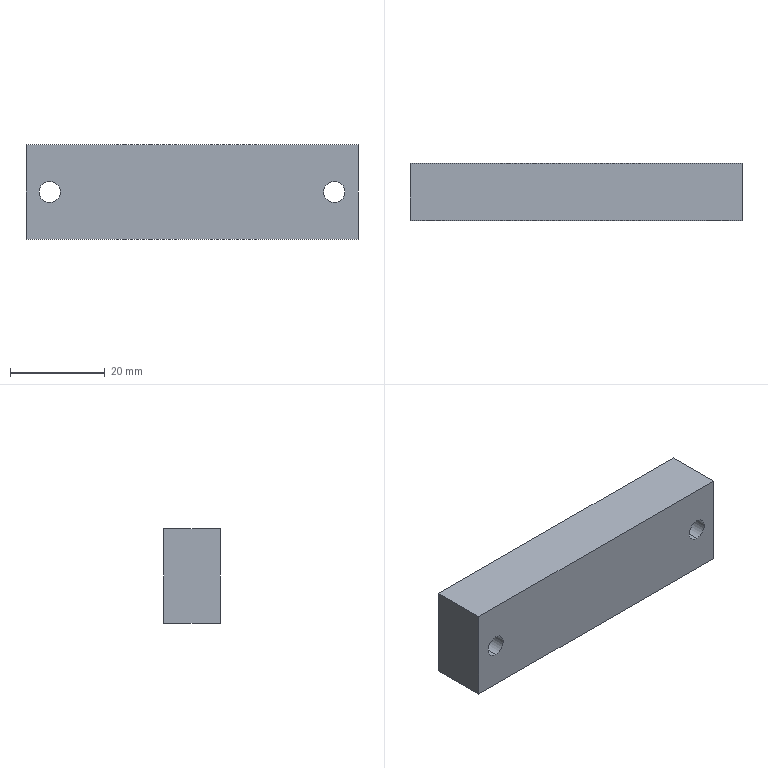Part | SolidWorks | features Extrusion 1, HoleWzd 1 | 1 solid | 16 faces | box 70 x 12 x 20 mm | volume 16291 mm3 | cylinder 8 | plane 8 | commonest cylinder face diameters 4.5 x4 7.8 x4
STEP:
#1=CARTESIAN_POINT('',(-30.,10.,-3.9));
#2=VERTEX_POINT('',#1);
#3=CARTESIAN_POINT('',(-30.,10.,3.9));
#4=VERTEX_POINT('',#3);
#5=CARTESIAN_POINT('',(-30.,10.,0.));
#6=DIRECTION('',(0.,1.,0.));
#7=DIRECTION('',(0.,0.,1.));
#8=AXIS2_PLACEMENT_3D('',#5,#6,#7);
#9=CIRCLE('',#8,3.9);
#10=EDGE_CURVE('',#2,#4,#9,.T.);
#11=ORIENTED_EDGE('',*,*,#10,.F.);
#12=CARTESIAN_POINT('',(-30.,12.,-3.9));
#13=VERTEX_POINT('',#12);
#14=CARTESIAN_POINT('',(-30.,12.,-3.9));
#15=DIRECTION('',(0.,1.,0.));
#16=VECTOR('',#15,1000.);
#17=LINE('',#14,#16);
#18=EDGE_CURVE('',#2,#13,#17,.T.);
#19=ORIENTED_EDGE('',*,*,#18,.T.);
#20=CARTESIAN_POINT('',(-30.,12.,3.9));
#21=VERTEX_POINT('',#20);
#22=CARTESIAN_POINT('',(-30.,12.,0.));
#23=DIRECTION('',(0.,1.,0.));
#24=DIRECTION('',(0.,0.,1.));
#25=AXIS2_PLACEMENT_3D('',#22,#23,#24);
#26=CIRCLE('',#25,3.9);
#27=EDGE_CURVE('',#13,#21,#26,.T.);
#28=ORIENTED_EDGE('',*,*,#27,.T.);
#29=CARTESIAN_POINT('',(-30.,12.,3.9));
#30=DIRECTION('',(0.,1.,0.));
#31=VECTOR('',#30,1000.);
#32=LINE('',#29,#31);
#33=EDGE_CURVE('',#4,#21,#32,.T.);
#34=ORIENTED_EDGE('',*,*,#33,.F.);
#35=EDGE_LOOP('',(#11,#19,#28,#34));
#36=FACE_OUTER_BOUND('',#35,.T.);
#37=CARTESIAN_POINT('',(-30.,12.,0.));
#38=DIRECTION('',(0.,1.,0.));
#39=DIRECTION('',(0.,0.,1.));
#40=AXIS2_PLACEMENT_3D('',#37,#38,#39);
#41=CYLINDRICAL_SURFACE('',#40,3.9);
#42=ADVANCED_FACE('',(#36),#41,.F.);
#43=CARTESIAN_POINT('',(-30.,0.,-2.25));
#44=VERTEX_POINT('',#43);
#45=CARTESIAN_POINT('',(-30.,0.,2.25));
#46=VERTEX_POINT('',#45);
#47=CARTESIAN_POINT('',(-30.,0.,0.));
#48=DIRECTION('',(0.,1.,0.));
#49=DIRECTION('',(0.,0.,1.));
#50=AXIS2_PLACEMENT_3D('',#47,#48,#49);
#51=CIRCLE('',#50,2.25);
#52=EDGE_CURVE('',#44,#46,#51,.T.);
#53=ORIENTED_EDGE('',*,*,#52,.F.);
#54=CARTESIAN_POINT('',(-30.,10.,-2.25));
#55=VERTEX_POINT('',#54);
#56=CARTESIAN_POINT('',(-30.,12.,-2.25));
#57=DIRECTION('',(0.,1.,0.));
#58=VECTOR('',#57,1000.);
#59=LINE('',#56,#58);
#60=EDGE_CURVE('',#44,#55,#59,.T.);
#61=ORIENTED_EDGE('',*,*,#60,.T.);
#62=CARTESIAN_POINT('',(-30.,10.,2.25));
#63=VERTEX_POINT('',#62);
#64=CARTESIAN_POINT('',(-30.,10.,0.));
#65=DIRECTION('',(0.,1.,0.));
#66=DIRECTION('',(0.,0.,1.));
#67=AXIS2_PLACEMENT_3D('',#64,#65,#66);
#68=CIRCLE('',#67,2.25);
#69=EDGE_CURVE('',#55,#63,#68,.T.);
#70=ORIENTED_EDGE('',*,*,#69,.T.);
#71=CARTESIAN_POINT('',(-30.,12.,2.25));
#72=DIRECTION('',(0.,1.,0.));
#73=VECTOR('',#72,1000.);
#74=LINE('',#71,#73);
#75=EDGE_CURVE('',#46,#63,#74,.T.);
#76=ORIENTED_EDGE('',*,*,#75,.F.);
#77=EDGE_LOOP('',(#53,#61,#70,#76));
#78=FACE_OUTER_BOUND('',#77,.T.);
#79=CARTESIAN_POINT('',(-30.,12.,0.));
#80=DIRECTION('',(0.,1.,0.));
#81=DIRECTION('',(0.,0.,1.));
#82=AXIS2_PLACEMENT_3D('',#79,#80,#81);
#83=CYLINDRICAL_SURFACE('',#82,2.25);
#84=ADVANCED_FACE('',(#78),#83,.F.);
#85=CARTESIAN_POINT('',(30.,10.,-3.9));
#86=VERTEX_POINT('',#85);
#87=CARTESIAN_POINT('',(30.,10.,3.9));
#88=VERTEX_POINT('',#87);
#89=CARTESIAN_POINT('',(30.,10.,0.));
#90=DIRECTION('',(0.,1.,0.));
#91=DIRECTION('',(0.,0.,1.));
#92=AXIS2_PLACEMENT_3D('',#89,#90,#91);
#93=CIRCLE('',#92,3.9);
#94=EDGE_CURVE('',#86,#88,#93,.T.);
#95=ORIENTED_EDGE('',*,*,#94,.F.);
#96=CARTESIAN_POINT('',(30.,12.,-3.9));
#97=VERTEX_POINT('',#96);
#98=CARTESIAN_POINT('',(30.,12.,-3.9));
#99=DIRECTION('',(0.,1.,0.));
#100=VECTOR('',#99,1000.);
#101=LINE('',#98,#100);
#102=EDGE_CURVE('',#86,#97,#101,.T.);
#103=ORIENTED_EDGE('',*,*,#102,.T.);
#104=CARTESIAN_POINT('',(30.,12.,3.9));
#105=VERTEX_POINT('',#104);
#106=CARTESIAN_POINT('',(30.,12.,0.));
#107=DIRECTION('',(0.,1.,0.));
#108=DIRECTION('',(0.,0.,1.));
#109=AXIS2_PLACEMENT_3D('',#106,#107,#108);
#110=CIRCLE('',#109,3.9);
#111=EDGE_CURVE('',#97,#105,#110,.T.);
#112=ORIENTED_EDGE('',*,*,#111,.T.);
#113=CARTESIAN_POINT('',(30.,12.,3.9));
#114=DIRECTION('',(0.,1.,0.));
#115=VECTOR('',#114,1000.);
#116=LINE('',#113,#115);
#117=EDGE_CURVE('',#88,#105,#116,.T.);
#118=ORIENTED_EDGE('',*,*,#117,.F.);
#119=EDGE_LOOP('',(#95,#103,#112,#118));
#120=FACE_OUTER_BOUND('',#119,.T.);
#121=CARTESIAN_POINT('',(30.,12.,0.));
#122=DIRECTION('',(0.,1.,0.));
#123=DIRECTION('',(0.,0.,1.));
#124=AXIS2_PLACEMENT_3D('',#121,#122,#123);
#125=CYLINDRICAL_SURFACE('',#124,3.9);
#126=ADVANCED_FACE('',(#120),#125,.F.);
#127=CARTESIAN_POINT('',(30.,0.,-2.25));
#128=VERTEX_POINT('',#127);
#129=CARTESIAN_POINT('',(30.,0.,2.25));
#130=VERTEX_POINT('',#129);
#131=CARTESIAN_POINT('',(30.,0.,0.));
#132=DIRECTION('',(0.,1.,0.));
#133=DIRECTION('',(0.,0.,1.));
#134=AXIS2_PLACEMENT_3D('',#131,#132,#133);
#135=CIRCLE('',#134,2.25);
#136=EDGE_CURVE('',#128,#130,#135,.T.);
#137=ORIENTED_EDGE('',*,*,#136,.F.);
#138=CARTESIAN_POINT('',(30.,10.,-2.25));
#139=VERTEX_POINT('',#138);
#140=CARTESIAN_POINT('',(30.,12.,-2.25));
#141=DIRECTION('',(0.,1.,0.));
#142=VECTOR('',#141,1000.);
#143=LINE('',#140,#142);
#144=EDGE_CURVE('',#128,#139,#143,.T.);
#145=ORIENTED_EDGE('',*,*,#144,.T.);
#146=CARTESIAN_POINT('',(30.,10.,2.25));
#147=VERTEX_POINT('',#146);
#148=CARTESIAN_POINT('',(30.,10.,0.));
#149=DIRECTION('',(0.,1.,0.));
#150=DIRECTION('',(0.,0.,1.));
#151=AXIS2_PLACEMENT_3D('',#148,#149,#150);
#152=CIRCLE('',#151,2.25);
#153=EDGE_CURVE('',#139,#147,#152,.T.);
#154=ORIENTED_EDGE('',*,*,#153,.T.);
#155=CARTESIAN_POINT('',(30.,12.,2.25));
#156=DIRECTION('',(0.,1.,0.));
#157=VECTOR('',#156,1000.);
#158=LINE('',#155,#157);
#159=EDGE_CURVE('',#130,#147,#158,.T.);
#160=ORIENTED_EDGE('',*,*,#159,.F.);
#161=EDGE_LOOP('',(#137,#145,#154,#160));
#162=FACE_OUTER_BOUND('',#161,.T.);
#163=CARTESIAN_POINT('',(30.,12.,0.));
#164=DIRECTION('',(0.,1.,0.));
#165=DIRECTION('',(0.,0.,1.));
#166=AXIS2_PLACEMENT_3D('',#163,#164,#165);
#167=CYLINDRICAL_SURFACE('',#166,2.25);
#168=ADVANCED_FACE('',(#162),#167,.F.);
#169=CARTESIAN_POINT('',(35.,0.,10.));
#170=VERTEX_POINT('',#169);
#171=CARTESIAN_POINT('',(35.,0.,-10.));
#172=VERTEX_POINT('',#171);
#173=CARTESIAN_POINT('',(35.,0.,-10.));
#174=DIRECTION('',(0.,0.,-1.));
#175=VECTOR('',#174,1000.);
#176=LINE('',#173,#175);
#177=EDGE_CURVE('',#170,#172,#176,.T.);
#178=ORIENTED_EDGE('',*,*,#177,.T.);
#179=CARTESIAN_POINT('',(35.,12.,-10.));
#180=VERTEX_POINT('',#179);
#181=CARTESIAN_POINT('',(35.,12.,-10.));
#182=DIRECTION('',(0.,-1.,0.));
#183=VECTOR('',#182,1000.);
#184=LINE('',#181,#183);
#185=EDGE_CURVE('',#180,#172,#184,.T.);
#186=ORIENTED_EDGE('',*,*,#185,.F.);
#187=CARTESIAN_POINT('',(35.,12.,10.));
#188=VERTEX_POINT('',#187);
#189=CARTESIAN_POINT('',(35.,12.,-10.));
#190=DIRECTION('',(0.,0.,-1.));
#191=VECTOR('',#190,1000.);
#192=LINE('',#189,#191);
#193=EDGE_CURVE('',#188,#180,#192,.T.);
#194=ORIENTED_EDGE('',*,*,#193,.F.);
#195=CARTESIAN_POINT('',(35.,12.,10.));
#196=DIRECTION('',(0.,-1.,0.));
#197=VECTOR('',#196,1000.);
#198=LINE('',#195,#197);
#199=EDGE_CURVE('',#188,#170,#198,.T.);
#200=ORIENTED_EDGE('',*,*,#199,.T.);
#201=EDGE_LOOP('',(#178,#186,#194,#200));
#202=FACE_OUTER_BOUND('',#201,.T.);
#203=CARTESIAN_POINT('',(35.,12.,-10.));
#204=DIRECTION('',(-1.,0.,0.));
#205=DIRECTION('',(0.,0.,1.));
#206=AXIS2_PLACEMENT_3D('',#203,#204,#205);
#207=PLANE('',#206);
#208=ADVANCED_FACE('',(#202),#207,.F.);
#209=CARTESIAN_POINT('',(-35.,0.,-10.));
#210=VERTEX_POINT('',#209);
#211=CARTESIAN_POINT('',(-35.,0.,-10.));
#212=DIRECTION('',(-1.,0.,0.));
#213=VECTOR('',#212,1000.);
#214=LINE('',#211,#213);
#215=EDGE_CURVE('',#172,#210,#214,.T.);
#216=ORIENTED_EDGE('',*,*,#215,.T.);
#217=CARTESIAN_POINT('',(-35.,12.,-10.));
#218=VERTEX_POINT('',#217);
#219=CARTESIAN_POINT('',(-35.,12.,-10.));
#220=DIRECTION('',(0.,-1.,0.));
#221=VECTOR('',#220,1000.);
#222=LINE('',#219,#221);
#223=EDGE_CURVE('',#218,#210,#222,.T.);
#224=ORIENTED_EDGE('',*,*,#223,.F.);
#225=CARTESIAN_POINT('',(-35.,12.,-10.));
#226=DIRECTION('',(-1.,0.,0.));
#227=VECTOR('',#226,1000.);
#228=LINE('',#225,#227);
#229=EDGE_CURVE('',#180,#218,#228,.T.);
#230=ORIENTED_EDGE('',*,*,#229,.F.);
#231=ORIENTED_EDGE('',*,*,#185,.T.);
#232=EDGE_LOOP('',(#216,#224,#230,#231));
#233=FACE_OUTER_BOUND('',#232,.T.);
#234=CARTESIAN_POINT('',(-35.,12.,-10.));
#235=DIRECTION('',(0.,0.,1.));
#236=DIRECTION('',(1.,0.,0.));
#237=AXIS2_PLACEMENT_3D('',#234,#235,#236);
#238=PLANE('',#237);
#239=ADVANCED_FACE('',(#233),#238,.F.);
#240=CARTESIAN_POINT('',(-35.,0.,10.));
#241=VERTEX_POINT('',#240);
#242=CARTESIAN_POINT('',(-35.,0.,-10.));
#243=DIRECTION('',(0.,0.,1.));
#244=VECTOR('',#243,1000.);
#245=LINE('',#242,#244);
#246=EDGE_CURVE('',#210,#241,#245,.T.);
#247=ORIENTED_EDGE('',*,*,#246,.T.);
#248=CARTESIAN_POINT('',(-35.,12.,10.));
#249=VERTEX_POINT('',#248);
#250=CARTESIAN_POINT('',(-35.,12.,10.));
#251=DIRECTION('',(0.,-1.,0.));
#252=VECTOR('',#251,1000.);
#253=LINE('',#250,#252);
#254=EDGE_CURVE('',#249,#241,#253,.T.);
#255=ORIENTED_EDGE('',*,*,#254,.F.);
#256=CARTESIAN_POINT('',(-35.,12.,-10.));
#257=DIRECTION('',(0.,0.,1.));
#258=VECTOR('',#257,1000.);
#259=LINE('',#256,#258);
#260=EDGE_CURVE('',#218,#249,#259,.T.);
#261=ORIENTED_EDGE('',*,*,#260,.F.);
#262=ORIENTED_EDGE('',*,*,#223,.T.);
#263=EDGE_LOOP('',(#247,#255,#261,#262));
#264=FACE_OUTER_BOUND('',#263,.T.);
#265=CARTESIAN_POINT('',(-35.,12.,-10.));
#266=DIRECTION('',(1.,0.,0.));
#267=DIRECTION('',(0.,0.,-1.));
#268=AXIS2_PLACEMENT_3D('',#265,#266,#267);
#269=PLANE('',#268);
#270=ADVANCED_FACE('',(#264),#269,.F.);
#271=CARTESIAN_POINT('',(-35.,0.,10.));
#272=DIRECTION('',(1.,0.,0.));
#273=VECTOR('',#272,1000.);
#274=LINE('',#271,#273);
#275=EDGE_CURVE('',#241,#170,#274,.T.);
#276=ORIENTED_EDGE('',*,*,#275,.T.);
#277=ORIENTED_EDGE('',*,*,#199,.F.);
#278=CARTESIAN_POINT('',(-35.,12.,10.));
#279=DIRECTION('',(1.,0.,0.));
#280=VECTOR('',#279,1000.);
#281=LINE('',#278,#280);
#282=EDGE_CURVE('',#249,#188,#281,.T.);
#283=ORIENTED_EDGE('',*,*,#282,.F.);
#284=ORIENTED_EDGE('',*,*,#254,.T.);
#285=EDGE_LOOP('',(#276,#277,#283,#284));
#286=FACE_OUTER_BOUND('',#285,.T.);
#287=CARTESIAN_POINT('',(-35.,12.,10.));
#288=DIRECTION('',(0.,0.,-1.));
#289=DIRECTION('',(-1.,0.,0.));
#290=AXIS2_PLACEMENT_3D('',#287,#288,#289);
#291=PLANE('',#290);
#292=ADVANCED_FACE('',(#286),#291,.F.);
#293=CARTESIAN_POINT('',(-30.,12.,0.));
#294=DIRECTION('',(0.,1.,0.));
#295=DIRECTION('',(0.,0.,1.));
#296=AXIS2_PLACEMENT_3D('',#293,#294,#295);
#297=CIRCLE('',#296,3.9);
#298=EDGE_CURVE('',#21,#13,#297,.T.);
#299=ORIENTED_EDGE('',*,*,#298,.F.);
#300=ORIENTED_EDGE('',*,*,#27,.F.);
#301=EDGE_LOOP('',(#299,#300));
#302=FACE_BOUND('',#301,.T.);
#303=CARTESIAN_POINT('',(30.,12.,0.));
#304=DIRECTION('',(0.,1.,0.));
#305=DIRECTION('',(0.,0.,1.));
#306=AXIS2_PLACEMENT_3D('',#303,#304,#305);
#307=CIRCLE('',#306,3.9);
#308=EDGE_CURVE('',#105,#97,#307,.T.);
#309=ORIENTED_EDGE('',*,*,#308,.F.);
#310=ORIENTED_EDGE('',*,*,#111,.F.);
#311=EDGE_LOOP('',(#309,#310));
#312=FACE_BOUND('',#311,.T.);
#313=ORIENTED_EDGE('',*,*,#193,.T.);
#314=ORIENTED_EDGE('',*,*,#229,.T.);
#315=ORIENTED_EDGE('',*,*,#260,.T.);
#316=ORIENTED_EDGE('',*,*,#282,.T.);
#317=EDGE_LOOP('',(#313,#314,#315,#316));
#318=FACE_OUTER_BOUND('',#317,.T.);
#319=CARTESIAN_POINT('',(0.,12.,0.));
#320=DIRECTION('',(0.,1.,0.));
#321=DIRECTION('',(0.,0.,1.));
#322=AXIS2_PLACEMENT_3D('',#319,#320,#321);
#323=PLANE('',#322);
#324=ADVANCED_FACE('',(#302,#312,#318),#323,.T.);
#325=CARTESIAN_POINT('',(-30.,0.,0.));
#326=DIRECTION('',(0.,1.,0.));
#327=DIRECTION('',(0.,0.,1.));
#328=AXIS2_PLACEMENT_3D('',#325,#326,#327);
#329=CIRCLE('',#328,2.25);
#330=EDGE_CURVE('',#46,#44,#329,.T.);
#331=ORIENTED_EDGE('',*,*,#330,.T.);
#332=ORIENTED_EDGE('',*,*,#52,.T.);
#333=EDGE_LOOP('',(#331,#332));
#334=FACE_BOUND('',#333,.T.);
#335=CARTESIAN_POINT('',(30.,0.,0.));
#336=DIRECTION('',(0.,1.,0.));
#337=DIRECTION('',(0.,0.,1.));
#338=AXIS2_PLACEMENT_3D('',#335,#336,#337);
#339=CIRCLE('',#338,2.25);
#340=EDGE_CURVE('',#130,#128,#339,.T.);
#341=ORIENTED_EDGE('',*,*,#340,.T.);
#342=ORIENTED_EDGE('',*,*,#136,.T.);
#343=EDGE_LOOP('',(#341,#342));
#344=FACE_BOUND('',#343,.T.);
#345=ORIENTED_EDGE('',*,*,#177,.F.);
#346=ORIENTED_EDGE('',*,*,#275,.F.);
#347=ORIENTED_EDGE('',*,*,#246,.F.);
#348=ORIENTED_EDGE('',*,*,#215,.F.);
#349=EDGE_LOOP('',(#345,#346,#347,#348));
#350=FACE_OUTER_BOUND('',#349,.T.);
#351=CARTESIAN_POINT('',(0.,0.,0.));
#352=DIRECTION('',(0.,1.,0.));
#353=DIRECTION('',(0.,0.,1.));
#354=AXIS2_PLACEMENT_3D('',#351,#352,#353);
#355=PLANE('',#354);
#356=ADVANCED_FACE('',(#334,#344,#350),#355,.F.);
#357=ORIENTED_EDGE('',*,*,#144,.F.);
#358=ORIENTED_EDGE('',*,*,#340,.F.);
#359=ORIENTED_EDGE('',*,*,#159,.T.);
#360=CARTESIAN_POINT('',(30.,10.,0.));
#361=DIRECTION('',(0.,1.,0.));
#362=DIRECTION('',(0.,0.,1.));
#363=AXIS2_PLACEMENT_3D('',#360,#361,#362);
#364=CIRCLE('',#363,2.25);
#365=EDGE_CURVE('',#147,#139,#364,.T.);
#366=ORIENTED_EDGE('',*,*,#365,.T.);
#367=EDGE_LOOP('',(#357,#358,#359,#366));
#368=FACE_OUTER_BOUND('',#367,.T.);
#369=CARTESIAN_POINT('',(30.,12.,0.));
#370=DIRECTION('',(0.,1.,0.));
#371=DIRECTION('',(0.,0.,1.));
#372=AXIS2_PLACEMENT_3D('',#369,#370,#371);
#373=CYLINDRICAL_SURFACE('',#372,2.25);
#374=ADVANCED_FACE('',(#368),#373,.F.);
#375=ORIENTED_EDGE('',*,*,#365,.F.);
#376=ORIENTED_EDGE('',*,*,#153,.F.);
#377=EDGE_LOOP('',(#375,#376));
#378=FACE_BOUND('',#377,.T.);
#379=CARTESIAN_POINT('',(30.,10.,0.));
#380=DIRECTION('',(0.,1.,0.));
#381=DIRECTION('',(0.,0.,1.));
#382=AXIS2_PLACEMENT_3D('',#379,#380,#381);
#383=CIRCLE('',#382,3.9);
#384=EDGE_CURVE('',#88,#86,#383,.T.);
#385=ORIENTED_EDGE('',*,*,#384,.T.);
#386=ORIENTED_EDGE('',*,*,#94,.T.);
#387=EDGE_LOOP('',(#385,#386));
#388=FACE_OUTER_BOUND('',#387,.T.);
#389=CARTESIAN_POINT('',(32.25,10.,0.));
#390=DIRECTION('',(0.,-1.,0.));
#391=DIRECTION('',(0.,0.,-1.));
#392=AXIS2_PLACEMENT_3D('',#389,#390,#391);
#393=PLANE('',#392);
#394=ADVANCED_FACE('',(#378,#388),#393,.F.);
#395=ORIENTED_EDGE('',*,*,#102,.F.);
#396=ORIENTED_EDGE('',*,*,#384,.F.);
#397=ORIENTED_EDGE('',*,*,#117,.T.);
#398=ORIENTED_EDGE('',*,*,#308,.T.);
#399=EDGE_LOOP('',(#395,#396,#397,#398));
#400=FACE_OUTER_BOUND('',#399,.T.);
#401=CARTESIAN_POINT('',(30.,12.,0.));
#402=DIRECTION('',(0.,1.,0.));
#403=DIRECTION('',(0.,0.,1.));
#404=AXIS2_PLACEMENT_3D('',#401,#402,#403);
#405=CYLINDRICAL_SURFACE('',#404,3.9);
#406=ADVANCED_FACE('',(#400),#405,.F.);
#407=ORIENTED_EDGE('',*,*,#60,.F.);
#408=ORIENTED_EDGE('',*,*,#330,.F.);
#409=ORIENTED_EDGE('',*,*,#75,.T.);
#410=CARTESIAN_POINT('',(-30.,10.,0.));
#411=DIRECTION('',(0.,1.,0.));
#412=DIRECTION('',(0.,0.,1.));
#413=AXIS2_PLACEMENT_3D('',#410,#411,#412);
#414=CIRCLE('',#413,2.25);
#415=EDGE_CURVE('',#63,#55,#414,.T.);
#416=ORIENTED_EDGE('',*,*,#415,.T.);
#417=EDGE_LOOP('',(#407,#408,#409,#416));
#418=FACE_OUTER_BOUND('',#417,.T.);
#419=CARTESIAN_POINT('',(-30.,12.,0.));
#420=DIRECTION('',(0.,1.,0.));
#421=DIRECTION('',(0.,0.,1.));
#422=AXIS2_PLACEMENT_3D('',#419,#420,#421);
#423=CYLINDRICAL_SURFACE('',#422,2.25);
#424=ADVANCED_FACE('',(#418),#423,.F.);
#425=ORIENTED_EDGE('',*,*,#415,.F.);
#426=ORIENTED_EDGE('',*,*,#69,.F.);
#427=EDGE_LOOP('',(#425,#426));
#428=FACE_BOUND('',#427,.T.);
#429=CARTESIAN_POINT('',(-30.,10.,0.));
#430=DIRECTION('',(0.,1.,0.));
#431=DIRECTION('',(0.,0.,1.));
#432=AXIS2_PLACEMENT_3D('',#429,#430,#431);
#433=CIRCLE('',#432,3.9);
#434=EDGE_CURVE('',#4,#2,#433,.T.);
#435=ORIENTED_EDGE('',*,*,#434,.T.);
#436=ORIENTED_EDGE('',*,*,#10,.T.);
#437=EDGE_LOOP('',(#435,#436));
#438=FACE_OUTER_BOUND('',#437,.T.);
#439=CARTESIAN_POINT('',(-27.75,10.,0.));
#440=DIRECTION('',(0.,-1.,0.));
#441=DIRECTION('',(0.,0.,-1.));
#442=AXIS2_PLACEMENT_3D('',#439,#440,#441);
#443=PLANE('',#442);
#444=ADVANCED_FACE('',(#428,#438),#443,.F.);
#445=ORIENTED_EDGE('',*,*,#18,.F.);
#446=ORIENTED_EDGE('',*,*,#434,.F.);
#447=ORIENTED_EDGE('',*,*,#33,.T.);
#448=ORIENTED_EDGE('',*,*,#298,.T.);
#449=EDGE_LOOP('',(#445,#446,#447,#448));
#450=FACE_OUTER_BOUND('',#449,.T.);
#451=CARTESIAN_POINT('',(-30.,12.,0.));
#452=DIRECTION('',(0.,1.,0.));
#453=DIRECTION('',(0.,0.,1.));
#454=AXIS2_PLACEMENT_3D('',#451,#452,#453);
#455=CYLINDRICAL_SURFACE('',#454,3.9);
#456=ADVANCED_FACE('',(#450),#455,.F.);
#457=CLOSED_SHELL('',(#42,#84,#126,#168,#208,#239,#270,#292,#324,#356,#374,#394,#406,#424,#444,#456));
#458=MANIFOLD_SOLID_BREP('',#457);
#459=CARTESIAN_POINT('',(0.,0.,0.));
#460=DIRECTION('',(0.,0.,1.));
#461=DIRECTION('',(1.,0.,0.));
#462=AXIS2_PLACEMENT_3D('',#459,#460,#461);
#463=(LENGTH_UNIT()NAMED_UNIT(*)SI_UNIT(.MILLI.,.METRE.));
#464=UNCERTAINTY_MEASURE_WITH_UNIT(LENGTH_MEASURE(0.00001),#463,'','');
#465=(NAMED_UNIT(*)PLANE_ANGLE_UNIT()SI_UNIT($,.RADIAN.));
#466=(NAMED_UNIT(*)SI_UNIT($,.STERADIAN.)SOLID_ANGLE_UNIT());
#467=(GEOMETRIC_REPRESENTATION_CONTEXT(3)GLOBAL_UNCERTAINTY_ASSIGNED_CONTEXT((#464))GLOBAL_UNIT_ASSIGNED_CONTEXT((#463,#465,#466))REPRESENTATION_CONTEXT('',''));
#468=ADVANCED_BREP_SHAPE_REPRESENTATION('',(#458,#462),#467);